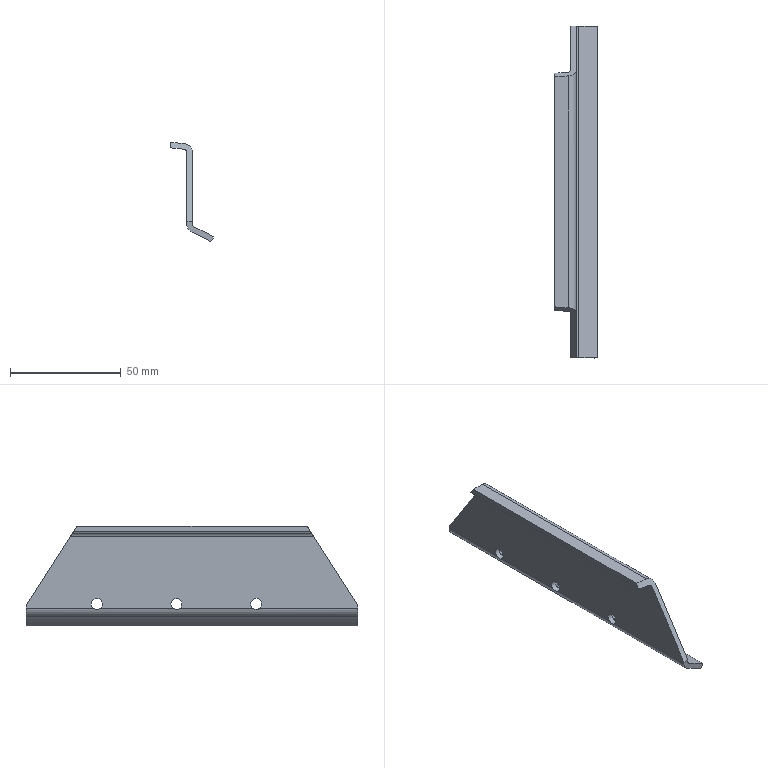Part | STEP file | 1-57.6 | 1 solid | 19 faces | box 19.684 x 150 x 44.877 mm | volume 17988 mm3 | cylinder 11 | plane 8 | commonest cylinder face diameters 5 x3 3 x2 8 x2 114 x1 119 x1 294 x1